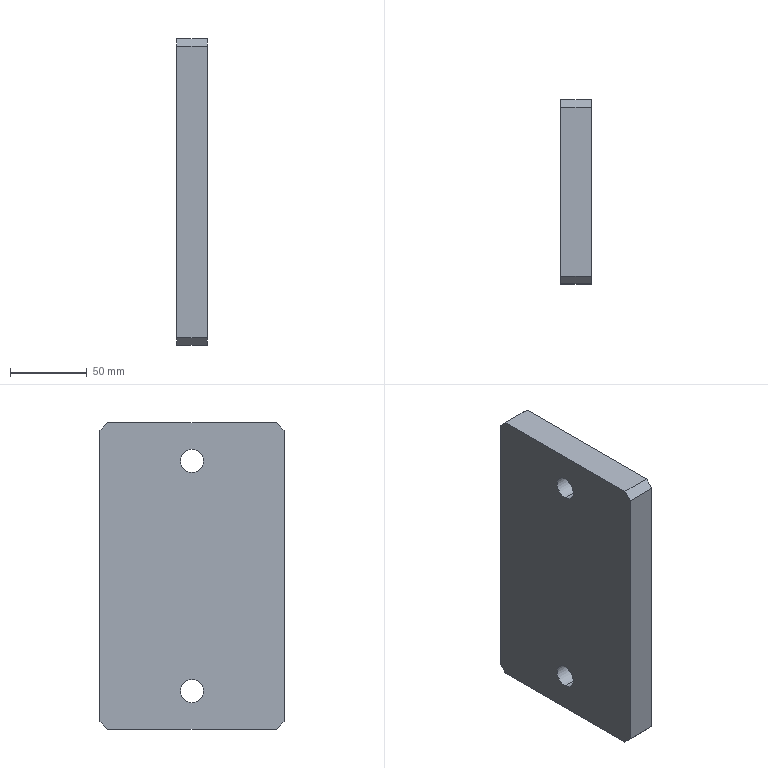Part | SolidWorks | features Chamfer 1, Extrusion 1, HoleWzd 1 | 1 solid | 14 faces | box 20 x 120 x 200 mm | volume 471931 mm3 | plane 10 | cylinder 4 | commonest cylinder face diameters 15 x4
STEP:
#1=CARTESIAN_POINT('',(0.,0.,82.5));
#2=VERTEX_POINT('',#1);
#3=CARTESIAN_POINT('',(0.,0.,67.5));
#4=VERTEX_POINT('',#3);
#5=CARTESIAN_POINT('',(0.,0.,75.));
#6=DIRECTION('',(1.,0.,0.));
#7=DIRECTION('',(0.,0.,-1.));
#8=AXIS2_PLACEMENT_3D('',#5,#6,#7);
#9=CIRCLE('',#8,7.5);
#10=EDGE_CURVE('',#2,#4,#9,.T.);
#11=ORIENTED_EDGE('',*,*,#10,.F.);
#12=CARTESIAN_POINT('',(20.,0.,82.5));
#13=VERTEX_POINT('',#12);
#14=CARTESIAN_POINT('',(20.,0.,82.5));
#15=DIRECTION('',(1.,0.,0.));
#16=VECTOR('',#15,1000.);
#17=LINE('',#14,#16);
#18=EDGE_CURVE('',#2,#13,#17,.T.);
#19=ORIENTED_EDGE('',*,*,#18,.T.);
#20=CARTESIAN_POINT('',(20.,0.,67.5));
#21=VERTEX_POINT('',#20);
#22=CARTESIAN_POINT('',(20.,0.,75.));
#23=DIRECTION('',(1.,0.,0.));
#24=DIRECTION('',(0.,0.,-1.));
#25=AXIS2_PLACEMENT_3D('',#22,#23,#24);
#26=CIRCLE('',#25,7.5);
#27=EDGE_CURVE('',#13,#21,#26,.T.);
#28=ORIENTED_EDGE('',*,*,#27,.T.);
#29=CARTESIAN_POINT('',(20.,0.,67.5));
#30=DIRECTION('',(1.,0.,0.));
#31=VECTOR('',#30,1000.);
#32=LINE('',#29,#31);
#33=EDGE_CURVE('',#4,#21,#32,.T.);
#34=ORIENTED_EDGE('',*,*,#33,.F.);
#35=EDGE_LOOP('',(#11,#19,#28,#34));
#36=FACE_OUTER_BOUND('',#35,.T.);
#37=CARTESIAN_POINT('',(20.,0.,75.));
#38=DIRECTION('',(1.,0.,0.));
#39=DIRECTION('',(0.,0.,-1.));
#40=AXIS2_PLACEMENT_3D('',#37,#38,#39);
#41=CYLINDRICAL_SURFACE('',#40,7.5);
#42=ADVANCED_FACE('',(#36),#41,.F.);
#43=CARTESIAN_POINT('',(0.,0.,-67.5));
#44=VERTEX_POINT('',#43);
#45=CARTESIAN_POINT('',(0.,0.,-82.5));
#46=VERTEX_POINT('',#45);
#47=CARTESIAN_POINT('',(0.,0.,-75.));
#48=DIRECTION('',(1.,0.,0.));
#49=DIRECTION('',(0.,0.,-1.));
#50=AXIS2_PLACEMENT_3D('',#47,#48,#49);
#51=CIRCLE('',#50,7.5);
#52=EDGE_CURVE('',#44,#46,#51,.T.);
#53=ORIENTED_EDGE('',*,*,#52,.F.);
#54=CARTESIAN_POINT('',(20.,0.,-67.5));
#55=VERTEX_POINT('',#54);
#56=CARTESIAN_POINT('',(20.,0.,-67.5));
#57=DIRECTION('',(1.,0.,0.));
#58=VECTOR('',#57,1000.);
#59=LINE('',#56,#58);
#60=EDGE_CURVE('',#44,#55,#59,.T.);
#61=ORIENTED_EDGE('',*,*,#60,.T.);
#62=CARTESIAN_POINT('',(20.,0.,-82.5));
#63=VERTEX_POINT('',#62);
#64=CARTESIAN_POINT('',(20.,0.,-75.));
#65=DIRECTION('',(1.,0.,0.));
#66=DIRECTION('',(0.,0.,-1.));
#67=AXIS2_PLACEMENT_3D('',#64,#65,#66);
#68=CIRCLE('',#67,7.5);
#69=EDGE_CURVE('',#55,#63,#68,.T.);
#70=ORIENTED_EDGE('',*,*,#69,.T.);
#71=CARTESIAN_POINT('',(20.,0.,-82.5));
#72=DIRECTION('',(1.,0.,0.));
#73=VECTOR('',#72,1000.);
#74=LINE('',#71,#73);
#75=EDGE_CURVE('',#46,#63,#74,.T.);
#76=ORIENTED_EDGE('',*,*,#75,.F.);
#77=EDGE_LOOP('',(#53,#61,#70,#76));
#78=FACE_OUTER_BOUND('',#77,.T.);
#79=CARTESIAN_POINT('',(20.,0.,-75.));
#80=DIRECTION('',(1.,0.,0.));
#81=DIRECTION('',(0.,0.,-1.));
#82=AXIS2_PLACEMENT_3D('',#79,#80,#81);
#83=CYLINDRICAL_SURFACE('',#82,7.5);
#84=ADVANCED_FACE('',(#78),#83,.F.);
#85=CARTESIAN_POINT('',(0.,-55.,-100.));
#86=VERTEX_POINT('',#85);
#87=CARTESIAN_POINT('',(0.,55.,-100.));
#88=VERTEX_POINT('',#87);
#89=CARTESIAN_POINT('',(0.,60.,-100.));
#90=DIRECTION('',(0.,1.,0.));
#91=VECTOR('',#90,1000.);
#92=LINE('',#89,#91);
#93=EDGE_CURVE('',#86,#88,#92,.T.);
#94=ORIENTED_EDGE('',*,*,#93,.T.);
#95=CARTESIAN_POINT('',(20.,55.,-100.));
#96=VERTEX_POINT('',#95);
#97=CARTESIAN_POINT('',(20.,55.,-100.));
#98=DIRECTION('',(1.,0.,0.));
#99=VECTOR('',#98,1000.);
#100=LINE('',#97,#99);
#101=EDGE_CURVE('',#88,#96,#100,.T.);
#102=ORIENTED_EDGE('',*,*,#101,.T.);
#103=CARTESIAN_POINT('',(20.,-55.,-100.));
#104=VERTEX_POINT('',#103);
#105=CARTESIAN_POINT('',(20.,60.,-100.));
#106=DIRECTION('',(0.,1.,0.));
#107=VECTOR('',#106,1000.);
#108=LINE('',#105,#107);
#109=EDGE_CURVE('',#104,#96,#108,.T.);
#110=ORIENTED_EDGE('',*,*,#109,.F.);
#111=CARTESIAN_POINT('',(20.,-55.,-100.));
#112=DIRECTION('',(-1.,0.,0.));
#113=VECTOR('',#112,1000.);
#114=LINE('',#111,#113);
#115=EDGE_CURVE('',#104,#86,#114,.T.);
#116=ORIENTED_EDGE('',*,*,#115,.T.);
#117=EDGE_LOOP('',(#94,#102,#110,#116));
#118=FACE_OUTER_BOUND('',#117,.T.);
#119=CARTESIAN_POINT('',(20.,60.,-100.));
#120=DIRECTION('',(0.,0.,1.));
#121=DIRECTION('',(0.,-1.,0.));
#122=AXIS2_PLACEMENT_3D('',#119,#120,#121);
#123=PLANE('',#122);
#124=ADVANCED_FACE('',(#118),#123,.F.);
#125=CARTESIAN_POINT('',(0.,60.,-95.));
#126=VERTEX_POINT('',#125);
#127=CARTESIAN_POINT('',(0.,60.,95.));
#128=VERTEX_POINT('',#127);
#129=CARTESIAN_POINT('',(0.,60.,100.));
#130=DIRECTION('',(0.,0.,1.));
#131=VECTOR('',#130,1000.);
#132=LINE('',#129,#131);
#133=EDGE_CURVE('',#126,#128,#132,.T.);
#134=ORIENTED_EDGE('',*,*,#133,.T.);
#135=CARTESIAN_POINT('',(20.,60.,95.));
#136=VERTEX_POINT('',#135);
#137=CARTESIAN_POINT('',(20.,60.,95.));
#138=DIRECTION('',(1.,0.,0.));
#139=VECTOR('',#138,1000.);
#140=LINE('',#137,#139);
#141=EDGE_CURVE('',#128,#136,#140,.T.);
#142=ORIENTED_EDGE('',*,*,#141,.T.);
#143=CARTESIAN_POINT('',(20.,60.,-95.));
#144=VERTEX_POINT('',#143);
#145=CARTESIAN_POINT('',(20.,60.,100.));
#146=DIRECTION('',(0.,0.,1.));
#147=VECTOR('',#146,1000.);
#148=LINE('',#145,#147);
#149=EDGE_CURVE('',#144,#136,#148,.T.);
#150=ORIENTED_EDGE('',*,*,#149,.F.);
#151=CARTESIAN_POINT('',(20.,60.,-95.));
#152=DIRECTION('',(-1.,0.,0.));
#153=VECTOR('',#152,1000.);
#154=LINE('',#151,#153);
#155=EDGE_CURVE('',#144,#126,#154,.T.);
#156=ORIENTED_EDGE('',*,*,#155,.T.);
#157=EDGE_LOOP('',(#134,#142,#150,#156));
#158=FACE_OUTER_BOUND('',#157,.T.);
#159=CARTESIAN_POINT('',(20.,60.,100.));
#160=DIRECTION('',(0.,-1.,0.));
#161=DIRECTION('',(0.,0.,-1.));
#162=AXIS2_PLACEMENT_3D('',#159,#160,#161);
#163=PLANE('',#162);
#164=ADVANCED_FACE('',(#158),#163,.F.);
#165=CARTESIAN_POINT('',(20.,55.,100.));
#166=VERTEX_POINT('',#165);
#167=CARTESIAN_POINT('',(20.,-55.,100.));
#168=VERTEX_POINT('',#167);
#169=CARTESIAN_POINT('',(20.,60.,100.));
#170=DIRECTION('',(0.,-1.,0.));
#171=VECTOR('',#170,1000.);
#172=LINE('',#169,#171);
#173=EDGE_CURVE('',#166,#168,#172,.T.);
#174=ORIENTED_EDGE('',*,*,#173,.F.);
#175=CARTESIAN_POINT('',(0.,55.,100.));
#176=VERTEX_POINT('',#175);
#177=CARTESIAN_POINT('',(20.,55.,100.));
#178=DIRECTION('',(-1.,0.,0.));
#179=VECTOR('',#178,1000.);
#180=LINE('',#177,#179);
#181=EDGE_CURVE('',#166,#176,#180,.T.);
#182=ORIENTED_EDGE('',*,*,#181,.T.);
#183=CARTESIAN_POINT('',(0.,-55.,100.));
#184=VERTEX_POINT('',#183);
#185=CARTESIAN_POINT('',(0.,60.,100.));
#186=DIRECTION('',(0.,-1.,0.));
#187=VECTOR('',#186,1000.);
#188=LINE('',#185,#187);
#189=EDGE_CURVE('',#176,#184,#188,.T.);
#190=ORIENTED_EDGE('',*,*,#189,.T.);
#191=CARTESIAN_POINT('',(20.,-55.,100.));
#192=DIRECTION('',(1.,0.,0.));
#193=VECTOR('',#192,1000.);
#194=LINE('',#191,#193);
#195=EDGE_CURVE('',#184,#168,#194,.T.);
#196=ORIENTED_EDGE('',*,*,#195,.T.);
#197=EDGE_LOOP('',(#174,#182,#190,#196));
#198=FACE_OUTER_BOUND('',#197,.T.);
#199=CARTESIAN_POINT('',(20.,60.,100.));
#200=DIRECTION('',(0.,0.,-1.));
#201=DIRECTION('',(0.,1.,0.));
#202=AXIS2_PLACEMENT_3D('',#199,#200,#201);
#203=PLANE('',#202);
#204=ADVANCED_FACE('',(#198),#203,.F.);
#205=CARTESIAN_POINT('',(20.,-60.,95.));
#206=VERTEX_POINT('',#205);
#207=CARTESIAN_POINT('',(20.,-60.,-95.));
#208=VERTEX_POINT('',#207);
#209=CARTESIAN_POINT('',(20.,-60.,100.));
#210=DIRECTION('',(0.,0.,-1.));
#211=VECTOR('',#210,1000.);
#212=LINE('',#209,#211);
#213=EDGE_CURVE('',#206,#208,#212,.T.);
#214=ORIENTED_EDGE('',*,*,#213,.F.);
#215=CARTESIAN_POINT('',(0.,-60.,95.));
#216=VERTEX_POINT('',#215);
#217=CARTESIAN_POINT('',(20.,-60.,95.));
#218=DIRECTION('',(-1.,0.,0.));
#219=VECTOR('',#218,1000.);
#220=LINE('',#217,#219);
#221=EDGE_CURVE('',#206,#216,#220,.T.);
#222=ORIENTED_EDGE('',*,*,#221,.T.);
#223=CARTESIAN_POINT('',(0.,-60.,-95.));
#224=VERTEX_POINT('',#223);
#225=CARTESIAN_POINT('',(0.,-60.,100.));
#226=DIRECTION('',(0.,0.,-1.));
#227=VECTOR('',#226,1000.);
#228=LINE('',#225,#227);
#229=EDGE_CURVE('',#216,#224,#228,.T.);
#230=ORIENTED_EDGE('',*,*,#229,.T.);
#231=CARTESIAN_POINT('',(20.,-60.,-95.));
#232=DIRECTION('',(1.,0.,0.));
#233=VECTOR('',#232,1000.);
#234=LINE('',#231,#233);
#235=EDGE_CURVE('',#224,#208,#234,.T.);
#236=ORIENTED_EDGE('',*,*,#235,.T.);
#237=EDGE_LOOP('',(#214,#222,#230,#236));
#238=FACE_OUTER_BOUND('',#237,.T.);
#239=CARTESIAN_POINT('',(20.,-60.,100.));
#240=DIRECTION('',(0.,1.,0.));
#241=DIRECTION('',(0.,0.,1.));
#242=AXIS2_PLACEMENT_3D('',#239,#240,#241);
#243=PLANE('',#242);
#244=ADVANCED_FACE('',(#238),#243,.F.);
#245=CARTESIAN_POINT('',(20.,0.,75.));
#246=DIRECTION('',(1.,0.,0.));
#247=DIRECTION('',(0.,0.,-1.));
#248=AXIS2_PLACEMENT_3D('',#245,#246,#247);
#249=CIRCLE('',#248,7.5);
#250=EDGE_CURVE('',#21,#13,#249,.T.);
#251=ORIENTED_EDGE('',*,*,#250,.F.);
#252=ORIENTED_EDGE('',*,*,#27,.F.);
#253=EDGE_LOOP('',(#251,#252));
#254=FACE_BOUND('',#253,.T.);
#255=CARTESIAN_POINT('',(20.,0.,-75.));
#256=DIRECTION('',(1.,0.,0.));
#257=DIRECTION('',(0.,0.,-1.));
#258=AXIS2_PLACEMENT_3D('',#255,#256,#257);
#259=CIRCLE('',#258,7.5);
#260=EDGE_CURVE('',#63,#55,#259,.T.);
#261=ORIENTED_EDGE('',*,*,#260,.F.);
#262=ORIENTED_EDGE('',*,*,#69,.F.);
#263=EDGE_LOOP('',(#261,#262));
#264=FACE_BOUND('',#263,.T.);
#265=ORIENTED_EDGE('',*,*,#149,.T.);
#266=CARTESIAN_POINT('',(20.,77.5,77.5));
#267=DIRECTION('',(0.,-0.7071,0.7071));
#268=VECTOR('',#267,1000.);
#269=LINE('',#266,#268);
#270=EDGE_CURVE('',#136,#166,#269,.T.);
#271=ORIENTED_EDGE('',*,*,#270,.T.);
#272=ORIENTED_EDGE('',*,*,#173,.T.);
#273=CARTESIAN_POINT('',(20.,-77.5,77.5));
#274=DIRECTION('',(0.,-0.7071,-0.7071));
#275=VECTOR('',#274,1000.);
#276=LINE('',#273,#275);
#277=EDGE_CURVE('',#168,#206,#276,.T.);
#278=ORIENTED_EDGE('',*,*,#277,.T.);
#279=ORIENTED_EDGE('',*,*,#213,.T.);
#280=CARTESIAN_POINT('',(20.,-77.5,-77.5));
#281=DIRECTION('',(0.,0.7071,-0.7071));
#282=VECTOR('',#281,1000.);
#283=LINE('',#280,#282);
#284=EDGE_CURVE('',#208,#104,#283,.T.);
#285=ORIENTED_EDGE('',*,*,#284,.T.);
#286=ORIENTED_EDGE('',*,*,#109,.T.);
#287=CARTESIAN_POINT('',(20.,77.5,-77.5));
#288=DIRECTION('',(0.,0.7071,0.7071));
#289=VECTOR('',#288,1000.);
#290=LINE('',#287,#289);
#291=EDGE_CURVE('',#96,#144,#290,.T.);
#292=ORIENTED_EDGE('',*,*,#291,.T.);
#293=EDGE_LOOP('',(#265,#271,#272,#278,#279,#285,#286,#292));
#294=FACE_OUTER_BOUND('',#293,.T.);
#295=CARTESIAN_POINT('',(20.,0.,0.));
#296=DIRECTION('',(1.,0.,0.));
#297=DIRECTION('',(0.,0.,-1.));
#298=AXIS2_PLACEMENT_3D('',#295,#296,#297);
#299=PLANE('',#298);
#300=ADVANCED_FACE('',(#254,#264,#294),#299,.T.);
#301=CARTESIAN_POINT('',(0.,0.,75.));
#302=DIRECTION('',(1.,0.,0.));
#303=DIRECTION('',(0.,0.,-1.));
#304=AXIS2_PLACEMENT_3D('',#301,#302,#303);
#305=CIRCLE('',#304,7.5);
#306=EDGE_CURVE('',#4,#2,#305,.T.);
#307=ORIENTED_EDGE('',*,*,#306,.T.);
#308=ORIENTED_EDGE('',*,*,#10,.T.);
#309=EDGE_LOOP('',(#307,#308));
#310=FACE_BOUND('',#309,.T.);
#311=CARTESIAN_POINT('',(0.,0.,-75.));
#312=DIRECTION('',(1.,0.,0.));
#313=DIRECTION('',(0.,0.,-1.));
#314=AXIS2_PLACEMENT_3D('',#311,#312,#313);
#315=CIRCLE('',#314,7.5);
#316=EDGE_CURVE('',#46,#44,#315,.T.);
#317=ORIENTED_EDGE('',*,*,#316,.T.);
#318=ORIENTED_EDGE('',*,*,#52,.T.);
#319=EDGE_LOOP('',(#317,#318));
#320=FACE_BOUND('',#319,.T.);
#321=ORIENTED_EDGE('',*,*,#189,.F.);
#322=CARTESIAN_POINT('',(0.,55.,100.));
#323=DIRECTION('',(0.,0.7071,-0.7071));
#324=VECTOR('',#323,1000.);
#325=LINE('',#322,#324);
#326=EDGE_CURVE('',#176,#128,#325,.T.);
#327=ORIENTED_EDGE('',*,*,#326,.T.);
#328=ORIENTED_EDGE('',*,*,#133,.F.);
#329=CARTESIAN_POINT('',(0.,60.,-95.));
#330=DIRECTION('',(0.,-0.7071,-0.7071));
#331=VECTOR('',#330,1000.);
#332=LINE('',#329,#331);
#333=EDGE_CURVE('',#126,#88,#332,.T.);
#334=ORIENTED_EDGE('',*,*,#333,.T.);
#335=ORIENTED_EDGE('',*,*,#93,.F.);
#336=CARTESIAN_POINT('',(0.,-55.,-100.));
#337=DIRECTION('',(0.,-0.7071,0.7071));
#338=VECTOR('',#337,1000.);
#339=LINE('',#336,#338);
#340=EDGE_CURVE('',#86,#224,#339,.T.);
#341=ORIENTED_EDGE('',*,*,#340,.T.);
#342=ORIENTED_EDGE('',*,*,#229,.F.);
#343=CARTESIAN_POINT('',(0.,-60.,95.));
#344=DIRECTION('',(0.,0.7071,0.7071));
#345=VECTOR('',#344,1000.);
#346=LINE('',#343,#345);
#347=EDGE_CURVE('',#216,#184,#346,.T.);
#348=ORIENTED_EDGE('',*,*,#347,.T.);
#349=EDGE_LOOP('',(#321,#327,#328,#334,#335,#341,#342,#348));
#350=FACE_OUTER_BOUND('',#349,.T.);
#351=CARTESIAN_POINT('',(0.,0.,0.));
#352=DIRECTION('',(1.,0.,0.));
#353=DIRECTION('',(0.,0.,-1.));
#354=AXIS2_PLACEMENT_3D('',#351,#352,#353);
#355=PLANE('',#354);
#356=ADVANCED_FACE('',(#310,#320,#350),#355,.F.);
#357=ORIENTED_EDGE('',*,*,#60,.F.);
#358=ORIENTED_EDGE('',*,*,#316,.F.);
#359=ORIENTED_EDGE('',*,*,#75,.T.);
#360=ORIENTED_EDGE('',*,*,#260,.T.);
#361=EDGE_LOOP('',(#357,#358,#359,#360));
#362=FACE_OUTER_BOUND('',#361,.T.);
#363=CARTESIAN_POINT('',(20.,0.,-75.));
#364=DIRECTION('',(1.,0.,0.));
#365=DIRECTION('',(0.,0.,-1.));
#366=AXIS2_PLACEMENT_3D('',#363,#364,#365);
#367=CYLINDRICAL_SURFACE('',#366,7.5);
#368=ADVANCED_FACE('',(#362),#367,.F.);
#369=ORIENTED_EDGE('',*,*,#18,.F.);
#370=ORIENTED_EDGE('',*,*,#306,.F.);
#371=ORIENTED_EDGE('',*,*,#33,.T.);
#372=ORIENTED_EDGE('',*,*,#250,.T.);
#373=EDGE_LOOP('',(#369,#370,#371,#372));
#374=FACE_OUTER_BOUND('',#373,.T.);
#375=CARTESIAN_POINT('',(20.,0.,75.));
#376=DIRECTION('',(1.,0.,0.));
#377=DIRECTION('',(0.,0.,-1.));
#378=AXIS2_PLACEMENT_3D('',#375,#376,#377);
#379=CYLINDRICAL_SURFACE('',#378,7.5);
#380=ADVANCED_FACE('',(#374),#379,.F.);
#381=ORIENTED_EDGE('',*,*,#270,.F.);
#382=ORIENTED_EDGE('',*,*,#141,.F.);
#383=ORIENTED_EDGE('',*,*,#326,.F.);
#384=ORIENTED_EDGE('',*,*,#181,.F.);
#385=EDGE_LOOP('',(#381,#382,#383,#384));
#386=FACE_OUTER_BOUND('',#385,.T.);
#387=CARTESIAN_POINT('',(20.,55.,100.));
#388=DIRECTION('',(0.,-0.7071,-0.7071));
#389=DIRECTION('',(-1.,0.,0.));
#390=AXIS2_PLACEMENT_3D('',#387,#388,#389);
#391=PLANE('',#390);
#392=ADVANCED_FACE('',(#386),#391,.F.);
#393=ORIENTED_EDGE('',*,*,#277,.F.);
#394=ORIENTED_EDGE('',*,*,#195,.F.);
#395=ORIENTED_EDGE('',*,*,#347,.F.);
#396=ORIENTED_EDGE('',*,*,#221,.F.);
#397=EDGE_LOOP('',(#393,#394,#395,#396));
#398=FACE_OUTER_BOUND('',#397,.T.);
#399=CARTESIAN_POINT('',(20.,-60.,95.));
#400=DIRECTION('',(0.,0.7071,-0.7071));
#401=DIRECTION('',(-1.,0.,0.));
#402=AXIS2_PLACEMENT_3D('',#399,#400,#401);
#403=PLANE('',#402);
#404=ADVANCED_FACE('',(#398),#403,.F.);
#405=ORIENTED_EDGE('',*,*,#291,.F.);
#406=ORIENTED_EDGE('',*,*,#101,.F.);
#407=ORIENTED_EDGE('',*,*,#333,.F.);
#408=ORIENTED_EDGE('',*,*,#155,.F.);
#409=EDGE_LOOP('',(#405,#406,#407,#408));
#410=FACE_OUTER_BOUND('',#409,.T.);
#411=CARTESIAN_POINT('',(20.,60.,-95.));
#412=DIRECTION('',(0.,-0.7071,0.7071));
#413=DIRECTION('',(-1.,0.,0.));
#414=AXIS2_PLACEMENT_3D('',#411,#412,#413);
#415=PLANE('',#414);
#416=ADVANCED_FACE('',(#410),#415,.F.);
#417=ORIENTED_EDGE('',*,*,#284,.F.);
#418=ORIENTED_EDGE('',*,*,#235,.F.);
#419=ORIENTED_EDGE('',*,*,#340,.F.);
#420=ORIENTED_EDGE('',*,*,#115,.F.);
#421=EDGE_LOOP('',(#417,#418,#419,#420));
#422=FACE_OUTER_BOUND('',#421,.T.);
#423=CARTESIAN_POINT('',(20.,-55.,-100.));
#424=DIRECTION('',(0.,0.7071,0.7071));
#425=DIRECTION('',(-1.,0.,0.));
#426=AXIS2_PLACEMENT_3D('',#423,#424,#425);
#427=PLANE('',#426);
#428=ADVANCED_FACE('',(#422),#427,.F.);
#429=CLOSED_SHELL('',(#42,#84,#124,#164,#204,#244,#300,#356,#368,#380,#392,#404,#416,#428));
#430=MANIFOLD_SOLID_BREP('',#429);
#431=CARTESIAN_POINT('',(0.,0.,0.));
#432=DIRECTION('',(0.,0.,1.));
#433=DIRECTION('',(1.,0.,0.));
#434=AXIS2_PLACEMENT_3D('',#431,#432,#433);
#435=(LENGTH_UNIT()NAMED_UNIT(*)SI_UNIT(.MILLI.,.METRE.));
#436=UNCERTAINTY_MEASURE_WITH_UNIT(LENGTH_MEASURE(0.00001),#435,'','');
#437=(NAMED_UNIT(*)PLANE_ANGLE_UNIT()SI_UNIT($,.RADIAN.));
#438=(NAMED_UNIT(*)SI_UNIT($,.STERADIAN.)SOLID_ANGLE_UNIT());
#439=(GEOMETRIC_REPRESENTATION_CONTEXT(3)GLOBAL_UNCERTAINTY_ASSIGNED_CONTEXT((#436))GLOBAL_UNIT_ASSIGNED_CONTEXT((#435,#437,#438))REPRESENTATION_CONTEXT('',''));
#440=ADVANCED_BREP_SHAPE_REPRESENTATION('',(#430,#434),#439);